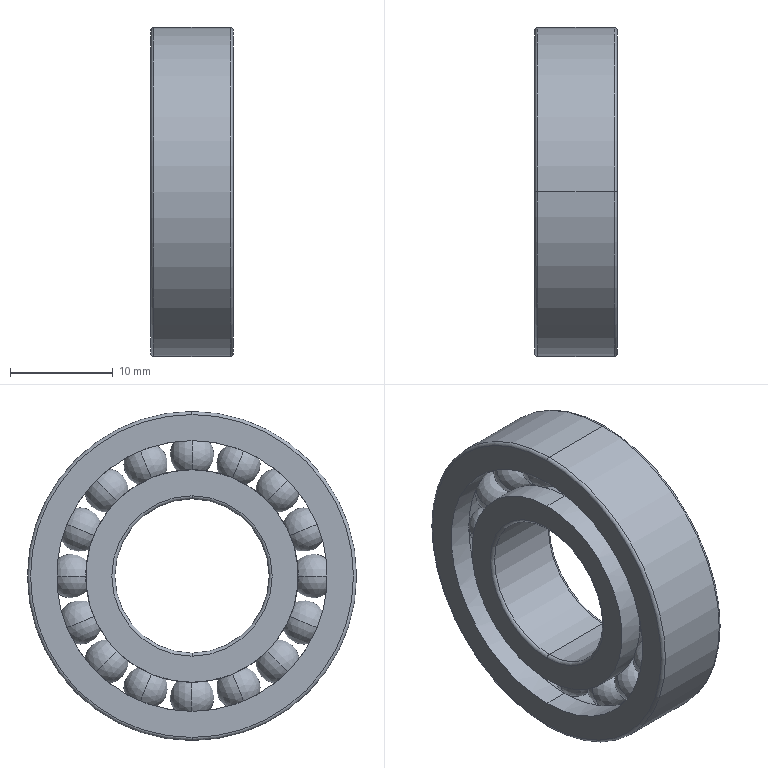Part | SolidWorks | features Revolution 3, CirPattern 1, Fillet 1 | 1 solid | 104 faces | box 8 x 32 x 32 mm | volume 3760 mm3 | torus 56 | sphere 32 | cylinder 12 | plane 4 | commonest cylinder face diameters 20.667 x4 26.333 x4 15 x2 32 x2